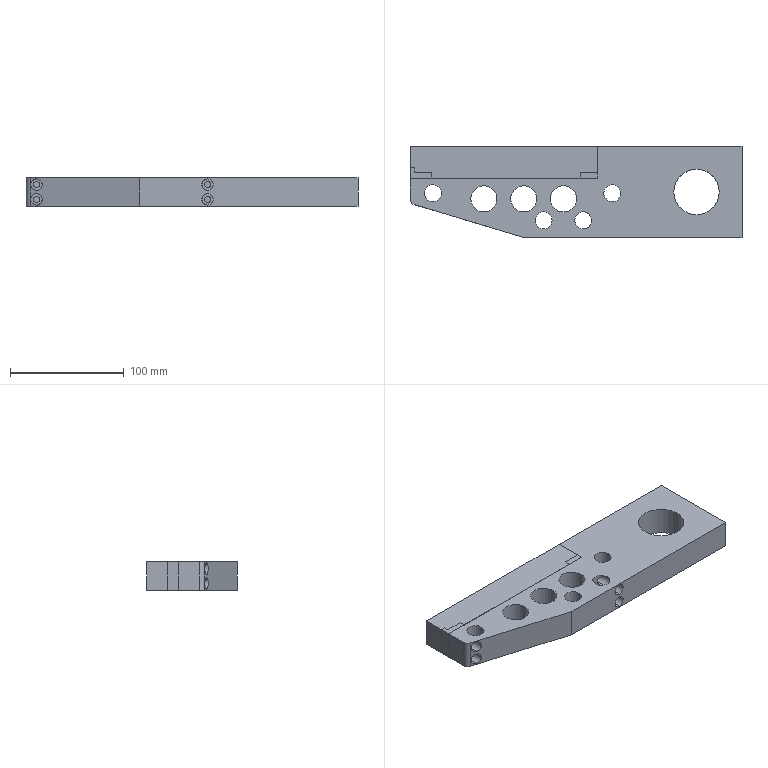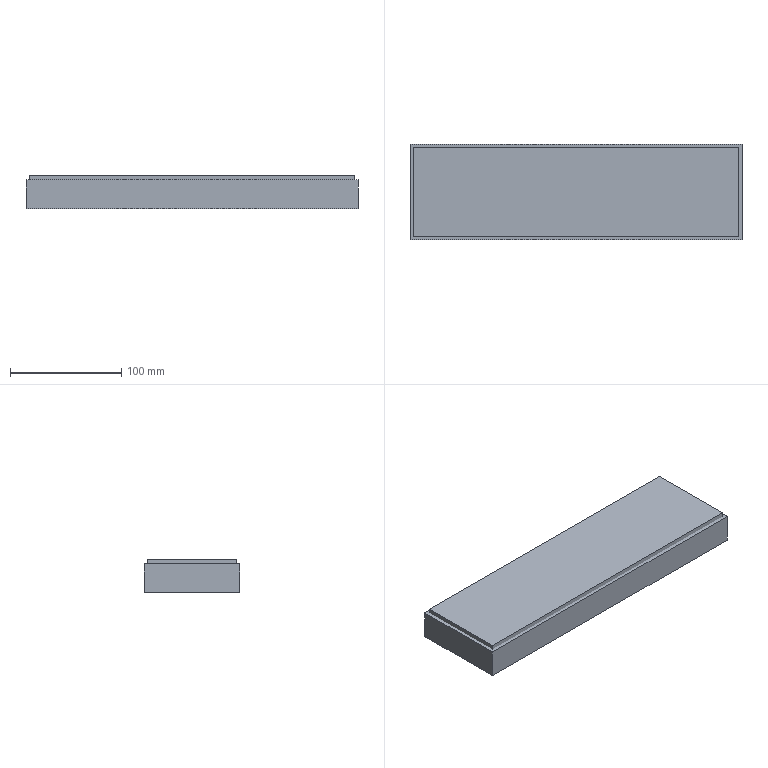CAM job | NX | 3-axis milling | part box 292 x 80 x 25 mm | stock box 298 x 86 x 30 mm
Tools:
number,name,description,diameter,corner_radius,flute_length,length,flutes
1,D50,Milling Tool-5 Parameters,50.0,0.0,50.0,75.0,2
3,D10,Milling Tool-5 Parameters,10.0,0.0,50.0,75.0,2
4,D10JING,Milling Tool-5 Parameters,10.0,0.0,50.0,75.0,2
2,D6A45,Milling Tool-5 Parameters,6.0,0.0,3.0,3.0,2
Operations:
program,operation,operation_type,tool,method,geometry_group,spindle_rpm,surface_speed,feed_per_tooth,feed_cut,feed_plunge,cut_length_mm,path_length_mm,cut_time_min,machine_time_min
1-295-85-30毛胚,FLOOR_WALL,VolumeBased25DMillingOperation,D50,METHOD,A,6500.0,1286.0,0.0962,1250.0,100.0,1121.997,1175.997,0.8976,0.903
1-295-85-30毛胚,ADAPTIVE_MILLING,CavityMilling,D10,METHOD,A,7000.0,219.0,0.1571,2200.0,1000.0,25491.703,29418.533,15.476,15.868
1-295-85-30毛胚,HOLE_MILLING,CylinderMilling,D10,METHOD,A,7000.0,131.0,0.1071,1500.0,100.0,2015.836,2524.265,1.344,1.395
1-295-85-30毛胚,ZLEVEL_PROFILE_COPY_COPY_1_COPY_COPY_COPY_1,ZLevelMilling,D10JING,METHOD,A,7000.0,219.0,0.0714,1000.0,100.0,2118.819,3919.396,2.119,2.299
1-295-85-30毛胚,ZLEVEL_PROFILE_COPY_1_COPY_COPY_COPY_COPY_2_COPY,ZLevelMilling,D6A45,METHOD,A,7000.0,131.0,0.0714,1000.0,1000.0,1237.478,2313.136,1.238,1.345
2-295-85-30毛胚,FLOOR_WALL_COPY,VolumeBased25DMillingOperation,D50,METHOD,B,6500.0,1286.0,0.0962,1250.0,100.0,5489.985,7152.522,4.392,4.558
2-295-85-30毛胚,ZLEVEL_PROFILE_COPY_1_COPY_COPY_COPY_COPY_2_COPY_COPY,ZLevelMilling,D6A45,METHOD,B,7000.0,131.0,0.0714,1000.0,1000.0,1237.635,2674.388,1.238,1.381